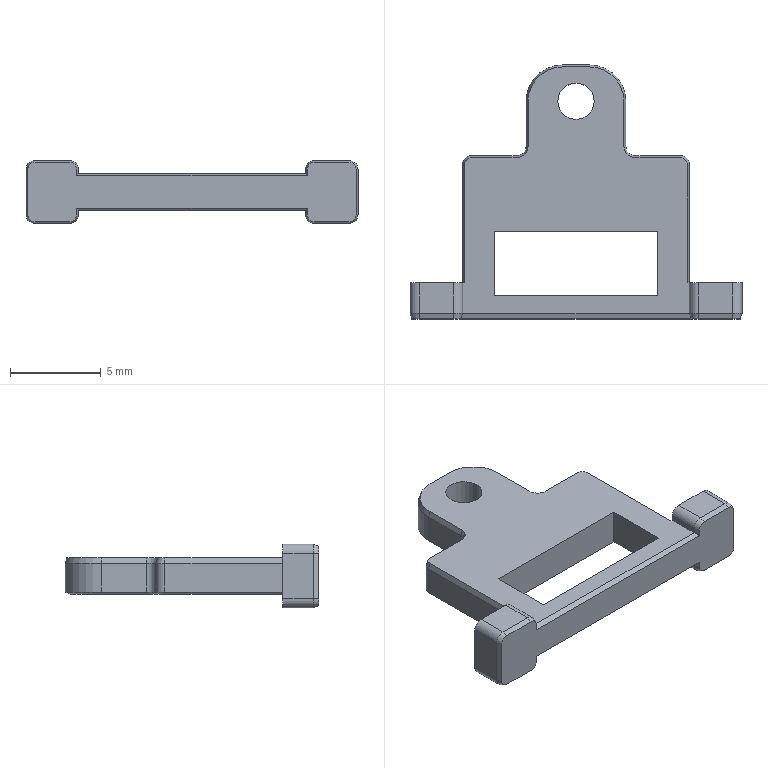Part | SolidWorks | features ICE 4, Attribute 3, Fillet 3, Chamfer 1, Extrusion 1, RefAxis 1 | 1 solid | 94 faces | box 18.3 x 14 x 3.5 mm | volume 236.065 mm3 | plane 54 | cylinder 20 | cone 20 | commonest cylinder face diameters 1 x12 2.2 x4 2 x2 4 x2